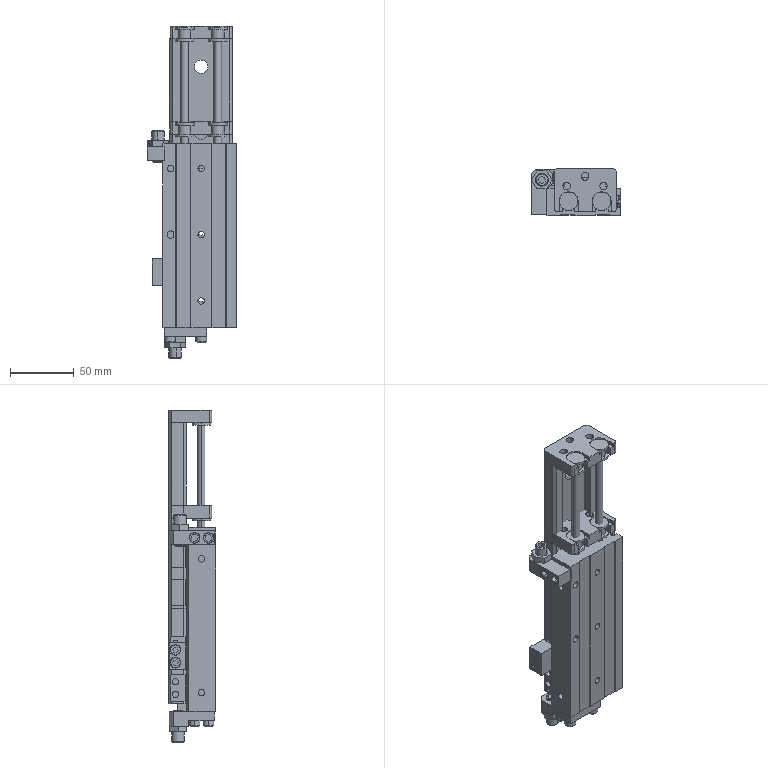Part | NX | 10 solids | 679 faces | box 70.6 x 37 x 260.875 mm | volume 365474 mm3 | plane 406 | cylinder 249 | cone 24 | commonest cylinder face diameters 5 x84 6 x24 8.5 x16 14.5 x16 10 x13 10.5 x12